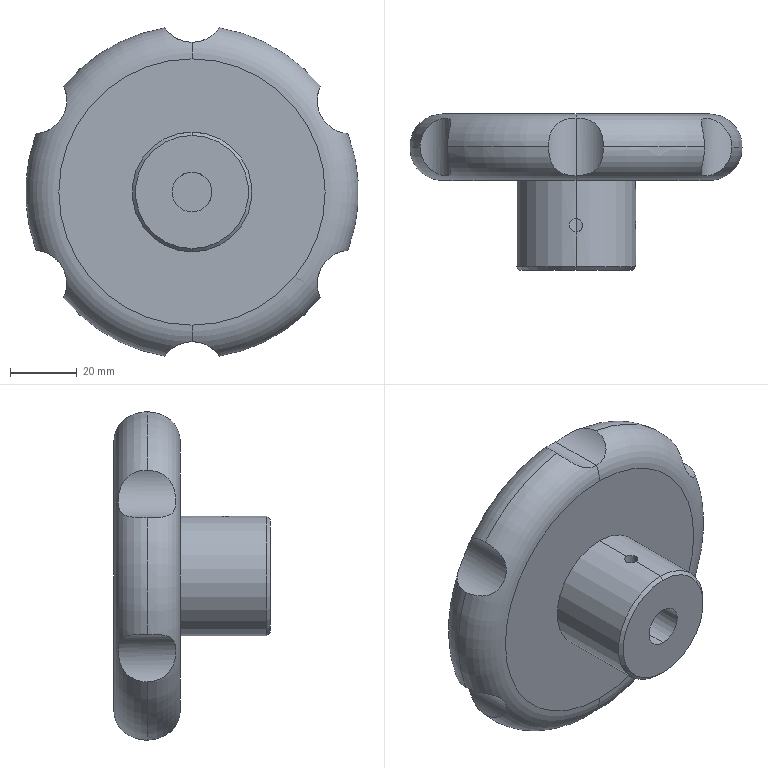Part | NX | features BREP 1 | 1 solid | 28 faces | box 100 x 47 x 98.636 mm | volume 156067 mm3 | cylinder 15 | plane 5 | cone 4 | torus 4 | commonest cylinder face diameters 20 x7 4 x4 12 x2 36 x2
STEP:
#1=CARTESIAN_POINT('',(0.,25.,6.));
#2=VERTEX_POINT('',#1);
#3=CARTESIAN_POINT('',(0.,25.,-6.));
#4=VERTEX_POINT('',#3);
#5=CARTESIAN_POINT('',(0.,25.,0.));
#6=DIRECTION('',(0.,-1.,0.));
#7=DIRECTION('',(0.,0.,1.));
#8=AXIS2_PLACEMENT_3D('',#5,#6,#7);
#9=CIRCLE('',#8,6.);
#10=EDGE_CURVE('',#2,#4,#9,.T.);
#11=ORIENTED_EDGE('',*,*,#10,.T.);
#12=CARTESIAN_POINT('',(0.,25.,0.));
#13=DIRECTION('',(0.,-1.,0.));
#14=DIRECTION('',(0.,0.,-1.));
#15=AXIS2_PLACEMENT_3D('',#12,#13,#14);
#16=CIRCLE('',#15,6.);
#17=EDGE_CURVE('',#4,#2,#16,.T.);
#18=ORIENTED_EDGE('',*,*,#17,.T.);
#19=EDGE_LOOP('',(#11,#18));
#20=FACE_BOUND('',#19,.T.);
#21=CARTESIAN_POINT('',(0.,25.,0.));
#22=DIRECTION('',(0.,1.,0.));
#23=DIRECTION('',(1.,0.,0.));
#24=AXIS2_PLACEMENT_3D('',#21,#22,#23);
#25=PLANE('',#24);
#26=ADVANCED_FACE('',(#20),#25,.F.);
#27=CARTESIAN_POINT('',(0.,0.,6.));
#28=VERTEX_POINT('',#27);
#29=CARTESIAN_POINT('',(0.,11.5,6.));
#30=VERTEX_POINT('',#29);
#31=CARTESIAN_POINT('',(0.,0.,6.));
#32=DIRECTION('',(0.,1.,0.));
#33=VECTOR('',#32,1000.);
#34=LINE('',#31,#33);
#35=EDGE_CURVE('',#28,#30,#34,.T.);
#36=ORIENTED_EDGE('',*,*,#35,.T.);
#37=CARTESIAN_POINT('',(2.,13.5,5.657));
#38=VERTEX_POINT('',#37);
#39=CARTESIAN_POINT('',(0.,11.5,6.));
#40=CARTESIAN_POINT('',(0.5281,11.5,6.));
#41=CARTESIAN_POINT('',(1.575,11.942,5.831));
#42=CARTESIAN_POINT('',(2.,12.98,5.657));
#43=CARTESIAN_POINT('',(2.,13.5,5.657));
#44=B_SPLINE_CURVE_WITH_KNOTS('',3,(#39,#40,#41,#42,#43),.UNSPECIFIED.,.F.,.F.,(4,1,4),(0.,0.5,1.),.UNSPECIFIED.);
#45=EDGE_CURVE('',#38,#30,#44,.F.);
#46=ORIENTED_EDGE('',*,*,#45,.F.);
#47=CARTESIAN_POINT('',(0.,15.5,6.));
#48=VERTEX_POINT('',#47);
#49=CARTESIAN_POINT('',(2.,13.5,5.657));
#50=CARTESIAN_POINT('',(2.,14.022,5.657));
#51=CARTESIAN_POINT('',(1.569,15.065,5.833));
#52=CARTESIAN_POINT('',(0.5245,15.5,6.));
#53=CARTESIAN_POINT('',(0.,15.5,6.));
#54=B_SPLINE_CURVE_WITH_KNOTS('',3,(#49,#50,#51,#52,#53),.UNSPECIFIED.,.F.,.F.,(4,1,4),(0.,0.5,1.),.UNSPECIFIED.);
#55=EDGE_CURVE('',#48,#38,#54,.F.);
#56=ORIENTED_EDGE('',*,*,#55,.F.);
#57=CARTESIAN_POINT('',(0.,15.5,6.));
#58=DIRECTION('',(0.,1.,0.));
#59=VECTOR('',#58,1000.);
#60=LINE('',#57,#59);
#61=EDGE_CURVE('',#2,#48,#60,.F.);
#62=ORIENTED_EDGE('',*,*,#61,.F.);
#63=ORIENTED_EDGE('',*,*,#17,.F.);
#64=CARTESIAN_POINT('',(0.,0.,-6.));
#65=VERTEX_POINT('',#64);
#66=CARTESIAN_POINT('',(0.,0.,-6.));
#67=DIRECTION('',(0.,1.,0.));
#68=VECTOR('',#67,1000.);
#69=LINE('',#66,#68);
#70=EDGE_CURVE('',#4,#65,#69,.F.);
#71=ORIENTED_EDGE('',*,*,#70,.T.);
#72=CARTESIAN_POINT('',(0.,0.,0.));
#73=DIRECTION('',(0.,1.,0.));
#74=DIRECTION('',(1.,0.,0.));
#75=AXIS2_PLACEMENT_3D('',#72,#73,#74);
#76=CIRCLE('',#75,6.);
#77=EDGE_CURVE('',#28,#65,#76,.T.);
#78=ORIENTED_EDGE('',*,*,#77,.F.);
#79=EDGE_LOOP('',(#36,#46,#56,#62,#63,#71,#78));
#80=FACE_BOUND('',#79,.T.);
#81=CARTESIAN_POINT('',(5.657,13.5,-2.));
#82=VERTEX_POINT('',#81);
#83=CARTESIAN_POINT('',(5.657,13.5,2.));
#84=VERTEX_POINT('',#83);
#85=CARTESIAN_POINT('',(5.657,13.5,2.));
#86=CARTESIAN_POINT('',(5.657,12.974,2.));
#87=CARTESIAN_POINT('',(5.836,11.924,1.555));
#88=CARTESIAN_POINT('',(6.083,11.283,0.006264));
#89=CARTESIAN_POINT('',(5.83,11.944,-1.582));
#90=CARTESIAN_POINT('',(5.657,12.981,-2.));
#91=CARTESIAN_POINT('',(5.657,13.5,-2.));
#92=B_SPLINE_CURVE_WITH_KNOTS('',3,(#85,#86,#87,#88,#89,#90,#91),.UNSPECIFIED.,.F.,.F.,(4,1,1,1,4),(0.,0.25,0.5,0.75,1.),.UNSPECIFIED.);
#93=EDGE_CURVE('',#82,#84,#92,.F.);
#94=ORIENTED_EDGE('',*,*,#93,.F.);
#95=CARTESIAN_POINT('',(5.657,13.5,-2.));
#96=CARTESIAN_POINT('',(5.657,14.,-2.));
#97=CARTESIAN_POINT('',(5.832,15.072,-1.572));
#98=CARTESIAN_POINT('',(6.083,15.714,-0.00285));
#99=CARTESIAN_POINT('',(5.834,15.071,1.564));
#100=CARTESIAN_POINT('',(5.657,14.024,2.));
#101=CARTESIAN_POINT('',(5.657,13.5,2.));
#102=B_SPLINE_CURVE_WITH_KNOTS('',3,(#95,#96,#97,#98,#99,#100,#101),.UNSPECIFIED.,.F.,.F.,(4,1,1,1,4),(0.,0.25,0.5,0.75,1.),.UNSPECIFIED.);
#103=EDGE_CURVE('',#84,#82,#102,.F.);
#104=ORIENTED_EDGE('',*,*,#103,.F.);
#105=EDGE_LOOP('',(#94,#104));
#106=FACE_BOUND('',#105,.T.);
#107=CARTESIAN_POINT('',(0.,25.,0.));
#108=DIRECTION('',(0.,1.,0.));
#109=DIRECTION('',(0.,0.,-1.));
#110=AXIS2_PLACEMENT_3D('',#107,#108,#109);
#111=CYLINDRICAL_SURFACE('',#110,6.);
#112=ADVANCED_FACE('',(#80,#106),#111,.F.);
#113=CARTESIAN_POINT('',(0.,0.,-17.));
#114=VERTEX_POINT('',#113);
#115=CARTESIAN_POINT('',(0.,0.,17.));
#116=VERTEX_POINT('',#115);
#117=CARTESIAN_POINT('',(0.,0.,0.));
#118=DIRECTION('',(0.,-1.,0.));
#119=DIRECTION('',(0.,0.,-1.));
#120=AXIS2_PLACEMENT_3D('',#117,#118,#119);
#121=CIRCLE('',#120,17.);
#122=EDGE_CURVE('',#114,#116,#121,.T.);
#123=ORIENTED_EDGE('',*,*,#122,.T.);
#124=CARTESIAN_POINT('',(0.,0.,0.));
#125=DIRECTION('',(0.,-1.,0.));
#126=DIRECTION('',(0.,0.,1.));
#127=AXIS2_PLACEMENT_3D('',#124,#125,#126);
#128=CIRCLE('',#127,17.);
#129=EDGE_CURVE('',#116,#114,#128,.T.);
#130=ORIENTED_EDGE('',*,*,#129,.T.);
#131=EDGE_LOOP('',(#123,#130));
#132=FACE_BOUND('',#131,.T.);
#133=CARTESIAN_POINT('',(0.,0.,0.));
#134=DIRECTION('',(0.,1.,0.));
#135=DIRECTION('',(0.,0.,-1.));
#136=AXIS2_PLACEMENT_3D('',#133,#134,#135);
#137=CIRCLE('',#136,6.);
#138=EDGE_CURVE('',#65,#28,#137,.T.);
#139=ORIENTED_EDGE('',*,*,#138,.T.);
#140=ORIENTED_EDGE('',*,*,#77,.T.);
#141=EDGE_LOOP('',(#139,#140));
#142=FACE_BOUND('',#141,.T.);
#143=CARTESIAN_POINT('',(0.,0.,0.));
#144=DIRECTION('',(0.,1.,0.));
#145=DIRECTION('',(1.,0.,0.));
#146=AXIS2_PLACEMENT_3D('',#143,#144,#145);
#147=PLANE('',#146);
#148=ADVANCED_FACE('',(#132,#142),#147,.F.);
#149=CARTESIAN_POINT('',(0.,1.,-18.));
#150=VERTEX_POINT('',#149);
#151=CARTESIAN_POINT('',(0.,0.,-17.));
#152=DIRECTION('',(0.,0.7071,-0.7071));
#153=VECTOR('',#152,1000.);
#154=LINE('',#151,#153);
#155=EDGE_CURVE('',#114,#150,#154,.T.);
#156=ORIENTED_EDGE('',*,*,#155,.F.);
#157=ORIENTED_EDGE('',*,*,#129,.F.);
#158=CARTESIAN_POINT('',(0.,1.,18.));
#159=VERTEX_POINT('',#158);
#160=CARTESIAN_POINT('',(0.,0.,17.));
#161=DIRECTION('',(0.,0.7071,0.7071));
#162=VECTOR('',#161,1000.);
#163=LINE('',#160,#162);
#164=EDGE_CURVE('',#116,#159,#163,.T.);
#165=ORIENTED_EDGE('',*,*,#164,.T.);
#166=CARTESIAN_POINT('',(0.,1.,0.));
#167=DIRECTION('',(0.,-1.,0.));
#168=DIRECTION('',(0.,0.,1.));
#169=AXIS2_PLACEMENT_3D('',#166,#167,#168);
#170=CIRCLE('',#169,18.);
#171=EDGE_CURVE('',#159,#150,#170,.T.);
#172=ORIENTED_EDGE('',*,*,#171,.T.);
#173=EDGE_LOOP('',(#156,#157,#165,#172));
#174=FACE_BOUND('',#173,.T.);
#175=CARTESIAN_POINT('',(0.,0.5,0.));
#176=DIRECTION('',(0.,1.,0.));
#177=DIRECTION('',(0.,0.,1.));
#178=AXIS2_PLACEMENT_3D('',#175,#176,#177);
#179=CONICAL_SURFACE('',#178,17.5,0.7854);
#180=ADVANCED_FACE('',(#174),#179,.T.);
#181=CARTESIAN_POINT('',(0.,11.5,18.));
#182=VERTEX_POINT('',#181);
#183=CARTESIAN_POINT('',(0.,11.5,18.));
#184=DIRECTION('',(0.,-1.,0.));
#185=VECTOR('',#184,1000.);
#186=LINE('',#183,#185);
#187=EDGE_CURVE('',#182,#159,#186,.T.);
#188=ORIENTED_EDGE('',*,*,#187,.F.);
#189=CARTESIAN_POINT('',(-2.,13.5,17.889));
#190=VERTEX_POINT('',#189);
#191=CARTESIAN_POINT('',(0.,11.5,18.));
#192=CARTESIAN_POINT('',(-1.065,11.5,18.));
#193=CARTESIAN_POINT('',(-1.999,12.443,17.889));
#194=CARTESIAN_POINT('',(-2.,13.5,17.889));
#195=B_SPLINE_CURVE_WITH_KNOTS('',3,(#191,#192,#193,#194),.UNSPECIFIED.,.F.,.F.,(4,4),(0.,1.),.UNSPECIFIED.);
#196=EDGE_CURVE('',#182,#190,#195,.T.);
#197=ORIENTED_EDGE('',*,*,#196,.T.);
#198=CARTESIAN_POINT('',(0.,15.5,18.));
#199=VERTEX_POINT('',#198);
#200=CARTESIAN_POINT('',(-2.,13.5,17.889));
#201=CARTESIAN_POINT('',(-1.999,14.557,17.889));
#202=CARTESIAN_POINT('',(-1.065,15.5,18.));
#203=CARTESIAN_POINT('',(0.,15.5,18.));
#204=B_SPLINE_CURVE_WITH_KNOTS('',3,(#200,#201,#202,#203),.UNSPECIFIED.,.F.,.F.,(4,4),(0.,1.),.UNSPECIFIED.);
#205=EDGE_CURVE('',#190,#199,#204,.T.);
#206=ORIENTED_EDGE('',*,*,#205,.T.);
#207=CARTESIAN_POINT('',(0.,27.,18.));
#208=VERTEX_POINT('',#207);
#209=CARTESIAN_POINT('',(0.,27.,18.));
#210=DIRECTION('',(0.,-1.,0.));
#211=VECTOR('',#210,1000.);
#212=LINE('',#209,#211);
#213=EDGE_CURVE('',#199,#208,#212,.F.);
#214=ORIENTED_EDGE('',*,*,#213,.T.);
#215=CARTESIAN_POINT('',(0.,27.,-18.));
#216=VERTEX_POINT('',#215);
#217=CARTESIAN_POINT('',(0.,27.,0.));
#218=DIRECTION('',(0.,1.,0.));
#219=DIRECTION('',(0.,0.,-1.));
#220=AXIS2_PLACEMENT_3D('',#217,#218,#219);
#221=CIRCLE('',#220,18.);
#222=EDGE_CURVE('',#216,#208,#221,.T.);
#223=ORIENTED_EDGE('',*,*,#222,.F.);
#224=CARTESIAN_POINT('',(0.,27.,-18.));
#225=DIRECTION('',(0.,-1.,0.));
#226=VECTOR('',#225,1000.);
#227=LINE('',#224,#226);
#228=EDGE_CURVE('',#150,#216,#227,.F.);
#229=ORIENTED_EDGE('',*,*,#228,.F.);
#230=ORIENTED_EDGE('',*,*,#171,.F.);
#231=EDGE_LOOP('',(#188,#197,#206,#214,#223,#229,#230));
#232=FACE_BOUND('',#231,.T.);
#233=CARTESIAN_POINT('',(0.,50.,0.));
#234=DIRECTION('',(0.,-1.,0.));
#235=DIRECTION('',(0.,0.,1.));
#236=AXIS2_PLACEMENT_3D('',#233,#234,#235);
#237=CYLINDRICAL_SURFACE('',#236,18.);
#238=ADVANCED_FACE('',(#232),#237,.T.);
#239=ORIENTED_EDGE('',*,*,#228,.T.);
#240=CARTESIAN_POINT('',(0.,27.,0.));
#241=DIRECTION('',(0.,1.,0.));
#242=DIRECTION('',(0.,0.,1.));
#243=AXIS2_PLACEMENT_3D('',#240,#241,#242);
#244=CIRCLE('',#243,18.);
#245=EDGE_CURVE('',#208,#216,#244,.T.);
#246=ORIENTED_EDGE('',*,*,#245,.F.);
#247=ORIENTED_EDGE('',*,*,#213,.F.);
#248=CARTESIAN_POINT('',(2.,13.5,17.889));
#249=VERTEX_POINT('',#248);
#250=CARTESIAN_POINT('',(0.,15.5,18.));
#251=CARTESIAN_POINT('',(1.057,15.5,18.));
#252=CARTESIAN_POINT('',(1.999,14.558,17.889));
#253=CARTESIAN_POINT('',(2.,13.5,17.889));
#254=B_SPLINE_CURVE_WITH_KNOTS('',3,(#250,#251,#252,#253),.UNSPECIFIED.,.F.,.F.,(4,4),(0.,1.),.UNSPECIFIED.);
#255=EDGE_CURVE('',#199,#249,#254,.T.);
#256=ORIENTED_EDGE('',*,*,#255,.T.);
#257=CARTESIAN_POINT('',(2.,13.5,17.889));
#258=CARTESIAN_POINT('',(1.999,12.44,17.889));
#259=CARTESIAN_POINT('',(1.061,11.5,18.));
#260=CARTESIAN_POINT('',(0.,11.5,18.));
#261=B_SPLINE_CURVE_WITH_KNOTS('',3,(#257,#258,#259,#260),.UNSPECIFIED.,.F.,.F.,(4,4),(0.,1.),.UNSPECIFIED.);
#262=EDGE_CURVE('',#249,#182,#261,.T.);
#263=ORIENTED_EDGE('',*,*,#262,.T.);
#264=ORIENTED_EDGE('',*,*,#187,.T.);
#265=CARTESIAN_POINT('',(0.,1.,0.));
#266=DIRECTION('',(0.,-1.,0.));
#267=DIRECTION('',(0.,0.,-1.));
#268=AXIS2_PLACEMENT_3D('',#265,#266,#267);
#269=CIRCLE('',#268,18.);
#270=EDGE_CURVE('',#150,#159,#269,.T.);
#271=ORIENTED_EDGE('',*,*,#270,.F.);
#272=EDGE_LOOP('',(#239,#246,#247,#256,#263,#264,#271));
#273=FACE_BOUND('',#272,.T.);
#274=CARTESIAN_POINT('',(17.889,13.5,2.));
#275=VERTEX_POINT('',#274);
#276=CARTESIAN_POINT('',(17.889,13.5,-2.));
#277=VERTEX_POINT('',#276);
#278=CARTESIAN_POINT('',(17.889,13.5,2.));
#279=CARTESIAN_POINT('',(17.889,14.03,2.));
#280=CARTESIAN_POINT('',(17.944,15.064,1.567));
#281=CARTESIAN_POINT('',(18.028,15.717,0.0006109));
#282=CARTESIAN_POINT('',(17.945,15.066,-1.564));
#283=CARTESIAN_POINT('',(17.889,14.031,-2.));
#284=CARTESIAN_POINT('',(17.889,13.5,-2.));
#285=B_SPLINE_CURVE_WITH_KNOTS('',3,(#278,#279,#280,#281,#282,#283,#284),.UNSPECIFIED.,.F.,.F.,(4,1,1,1,4),(0.,0.25,0.5,0.75,1.),.UNSPECIFIED.);
#286=EDGE_CURVE('',#275,#277,#285,.T.);
#287=ORIENTED_EDGE('',*,*,#286,.T.);
#288=CARTESIAN_POINT('',(17.889,13.5,-2.));
#289=CARTESIAN_POINT('',(17.889,12.967,-2.));
#290=CARTESIAN_POINT('',(17.945,11.93,-1.56));
#291=CARTESIAN_POINT('',(18.027,11.288,-0.005678));
#292=CARTESIAN_POINT('',(17.946,11.917,1.549));
#293=CARTESIAN_POINT('',(17.889,12.965,2.));
#294=CARTESIAN_POINT('',(17.889,13.5,2.));
#295=B_SPLINE_CURVE_WITH_KNOTS('',3,(#288,#289,#290,#291,#292,#293,#294),.UNSPECIFIED.,.F.,.F.,(4,1,1,1,4),(0.,0.25,0.5,0.75,1.),.UNSPECIFIED.);
#296=EDGE_CURVE('',#277,#275,#295,.T.);
#297=ORIENTED_EDGE('',*,*,#296,.T.);
#298=EDGE_LOOP('',(#287,#297));
#299=FACE_BOUND('',#298,.T.);
#300=CARTESIAN_POINT('',(0.,50.,0.));
#301=DIRECTION('',(0.,-1.,0.));
#302=DIRECTION('',(0.,0.,1.));
#303=AXIS2_PLACEMENT_3D('',#300,#301,#302);
#304=CYLINDRICAL_SURFACE('',#303,18.);
#305=ADVANCED_FACE('',(#273,#299),#304,.T.);
#306=ORIENTED_EDGE('',*,*,#164,.F.);
#307=ORIENTED_EDGE('',*,*,#122,.F.);
#308=ORIENTED_EDGE('',*,*,#155,.T.);
#309=ORIENTED_EDGE('',*,*,#270,.T.);
#310=EDGE_LOOP('',(#306,#307,#308,#309));
#311=FACE_BOUND('',#310,.T.);
#312=CARTESIAN_POINT('',(0.,0.5,0.));
#313=DIRECTION('',(0.,1.,0.));
#314=DIRECTION('',(0.,0.,1.));
#315=AXIS2_PLACEMENT_3D('',#312,#313,#314);
#316=CONICAL_SURFACE('',#315,17.5,0.7854);
#317=ADVANCED_FACE('',(#311),#316,.T.);
#318=CARTESIAN_POINT('',(-2.,13.5,5.657));
#319=VERTEX_POINT('',#318);
#320=CARTESIAN_POINT('',(0.,11.5,6.));
#321=CARTESIAN_POINT('',(-0.2457,11.5,6.));
#322=CARTESIAN_POINT('',(-0.6324,11.564,5.977));
#323=CARTESIAN_POINT('',(-1.071,11.805,5.905));
#324=CARTESIAN_POINT('',(-1.233,11.922,5.872));
#325=CARTESIAN_POINT('',(-1.411,12.073,5.833));
#326=CARTESIAN_POINT('',(-1.587,12.278,5.787));
#327=CARTESIAN_POINT('',(-1.68,12.408,5.76));
#328=CARTESIAN_POINT('',(-1.942,12.869,5.68));
#329=CARTESIAN_POINT('',(-2.,13.255,5.657));
#330=CARTESIAN_POINT('',(-2.,13.5,5.657));
#331=B_SPLINE_CURVE_WITH_KNOTS('',3,(#320,#321,#322,#323,#324,#325,#326,#327,#328,#329,#330),.UNSPECIFIED.,.F.,.F.,(4,1,1,1,1,1,1,1,4),(0.,0.25,0.375,0.4375,0.5,0.5625,0.625,0.75,1.),.UNSPECIFIED.);
#332=EDGE_CURVE('',#30,#319,#331,.T.);
#333=ORIENTED_EDGE('',*,*,#332,.T.);
#334=CARTESIAN_POINT('',(-2.,13.5,17.889));
#335=DIRECTION('',(0.,0.,-1.));
#336=VECTOR('',#335,1000.);
#337=LINE('',#334,#336);
#338=EDGE_CURVE('',#190,#319,#337,.T.);
#339=ORIENTED_EDGE('',*,*,#338,.F.);
#340=ORIENTED_EDGE('',*,*,#196,.F.);
#341=ORIENTED_EDGE('',*,*,#262,.F.);
#342=CARTESIAN_POINT('',(2.,13.5,17.889));
#343=DIRECTION('',(0.,0.,-1.));
#344=VECTOR('',#343,1000.);
#345=LINE('',#342,#344);
#346=EDGE_CURVE('',#249,#38,#345,.T.);
#347=ORIENTED_EDGE('',*,*,#346,.T.);
#348=ORIENTED_EDGE('',*,*,#45,.T.);
#349=EDGE_LOOP('',(#333,#339,#340,#341,#347,#348));
#350=FACE_BOUND('',#349,.T.);
#351=CARTESIAN_POINT('',(0.,13.5,18.));
#352=DIRECTION('',(0.,0.,-1.));
#353=DIRECTION('',(1.,0.,0.));
#354=AXIS2_PLACEMENT_3D('',#351,#352,#353);
#355=CYLINDRICAL_SURFACE('',#354,2.);
#356=ADVANCED_FACE('',(#350),#355,.F.);
#357=ORIENTED_EDGE('',*,*,#55,.T.);
#358=ORIENTED_EDGE('',*,*,#346,.F.);
#359=ORIENTED_EDGE('',*,*,#255,.F.);
#360=ORIENTED_EDGE('',*,*,#205,.F.);
#361=ORIENTED_EDGE('',*,*,#338,.T.);
#362=CARTESIAN_POINT('',(-2.,13.5,5.657));
#363=CARTESIAN_POINT('',(-2.,13.744,5.657));
#364=CARTESIAN_POINT('',(-1.941,14.129,5.68));
#365=CARTESIAN_POINT('',(-1.685,14.584,5.759));
#366=CARTESIAN_POINT('',(-1.589,14.719,5.786));
#367=CARTESIAN_POINT('',(-1.417,14.92,5.831));
#368=CARTESIAN_POINT('',(-1.237,15.075,5.871));
#369=CARTESIAN_POINT('',(-1.078,15.191,5.904));
#370=CARTESIAN_POINT('',(-0.637,15.435,5.977));
#371=CARTESIAN_POINT('',(-0.2473,15.5,6.));
#372=CARTESIAN_POINT('',(0.,15.5,6.));
#373=B_SPLINE_CURVE_WITH_KNOTS('',3,(#362,#363,#364,#365,#366,#367,#368,#369,#370,#371,#372),.UNSPECIFIED.,.F.,.F.,(4,1,1,1,1,1,1,1,4),(0.,0.25,0.375,0.4375,0.5,0.5625,0.625,0.75,1.),.UNSPECIFIED.);
#374=EDGE_CURVE('',#319,#48,#373,.T.);
#375=ORIENTED_EDGE('',*,*,#374,.T.);
#376=EDGE_LOOP('',(#357,#358,#359,#360,#361,#375));
#377=FACE_BOUND('',#376,.T.);
#378=CARTESIAN_POINT('',(0.,13.5,18.));
#379=DIRECTION('',(0.,0.,-1.));
#380=DIRECTION('',(1.,0.,0.));
#381=AXIS2_PLACEMENT_3D('',#378,#379,#380);
#382=CYLINDRICAL_SURFACE('',#381,2.);
#383=ADVANCED_FACE('',(#377),#382,.F.);
#384=ORIENTED_EDGE('',*,*,#138,.F.);
#385=ORIENTED_EDGE('',*,*,#70,.F.);
#386=ORIENTED_EDGE('',*,*,#10,.F.);
#387=ORIENTED_EDGE('',*,*,#61,.T.);
#388=ORIENTED_EDGE('',*,*,#374,.F.);
#389=ORIENTED_EDGE('',*,*,#332,.F.);
#390=ORIENTED_EDGE('',*,*,#35,.F.);
#391=EDGE_LOOP('',(#384,#385,#386,#387,#388,#389,#390));
#392=FACE_BOUND('',#391,.T.);
#393=CARTESIAN_POINT('',(0.,25.,0.));
#394=DIRECTION('',(0.,1.,0.));
#395=DIRECTION('',(0.,0.,-1.));
#396=AXIS2_PLACEMENT_3D('',#393,#394,#395);
#397=CYLINDRICAL_SURFACE('',#396,6.);
#398=ADVANCED_FACE('',(#392),#397,.F.);
#399=CARTESIAN_POINT('',(0.,27.,-40.));
#400=VERTEX_POINT('',#399);
#401=CARTESIAN_POINT('',(0.,27.,40.));
#402=VERTEX_POINT('',#401);
#403=CARTESIAN_POINT('',(0.,27.,0.));
#404=DIRECTION('',(0.,-1.,0.));
#405=DIRECTION('',(0.,0.,-1.));
#406=AXIS2_PLACEMENT_3D('',#403,#404,#405);
#407=CIRCLE('',#406,40.);
#408=EDGE_CURVE('',#400,#402,#407,.T.);
#409=ORIENTED_EDGE('',*,*,#408,.T.);
#410=CARTESIAN_POINT('',(0.,27.,0.));
#411=DIRECTION('',(0.,-1.,0.));
#412=DIRECTION('',(0.,0.,1.));
#413=AXIS2_PLACEMENT_3D('',#410,#411,#412);
#414=CIRCLE('',#413,40.);
#415=EDGE_CURVE('',#402,#400,#414,.T.);
#416=ORIENTED_EDGE('',*,*,#415,.T.);
#417=EDGE_LOOP('',(#409,#416));
#418=FACE_BOUND('',#417,.T.);
#419=ORIENTED_EDGE('',*,*,#222,.T.);
#420=ORIENTED_EDGE('',*,*,#245,.T.);
#421=EDGE_LOOP('',(#419,#420));
#422=FACE_BOUND('',#421,.T.);
#423=CARTESIAN_POINT('',(0.,27.,18.));
#424=DIRECTION('',(0.,1.,0.));
#425=DIRECTION('',(1.,0.,0.));
#426=AXIS2_PLACEMENT_3D('',#423,#424,#425);
#427=PLANE('',#426);
#428=ADVANCED_FACE('',(#418,#422),#427,.F.);
#429=CARTESIAN_POINT('',(0.,28.34,45.));
#430=VERTEX_POINT('',#429);
#431=CARTESIAN_POINT('',(0.,37.,40.));
#432=DIRECTION('',(-1.,0.,0.));
#433=DIRECTION('',(0.,-1.,0.));
#434=AXIS2_PLACEMENT_3D('',#431,#432,#433);
#435=CIRCLE('',#434,10.);
#436=EDGE_CURVE('',#430,#402,#435,.F.);
#437=ORIENTED_EDGE('',*,*,#436,.F.);
#438=CARTESIAN_POINT('',(-5.837,30.104,46.88));
#439=VERTEX_POINT('',#438);
#440=CARTESIAN_POINT('',(-5.837,30.104,46.88));
#441=CARTESIAN_POINT('',(-5.144,29.495,46.382));
#442=CARTESIAN_POINT('',(-3.305,28.575,45.374));
#443=CARTESIAN_POINT('',(-1.125,28.34,45.));
#444=CARTESIAN_POINT('',(0.,28.34,45.));
#445=B_SPLINE_CURVE_WITH_KNOTS('',3,(#440,#441,#442,#443,#444),.UNSPECIFIED.,.F.,.F.,(4,1,4),(0.,0.5,1.),.UNSPECIFIED.);
#446=EDGE_CURVE('',#430,#439,#445,.F.);
#447=ORIENTED_EDGE('',*,*,#446,.T.);
#448=CARTESIAN_POINT('',(-8.229,37.,49.318));
#449=VERTEX_POINT('',#448);
#450=CARTESIAN_POINT('',(-8.229,37.,49.318));
#451=CARTESIAN_POINT('',(-8.229,35.555,49.318));
#452=CARTESIAN_POINT('',(-7.84,32.733,48.706));
#453=CARTESIAN_POINT('',(-6.663,30.83,47.474));
#454=CARTESIAN_POINT('',(-5.837,30.104,46.88));
#455=B_SPLINE_CURVE_WITH_KNOTS('',3,(#450,#451,#452,#453,#454),.UNSPECIFIED.,.F.,.F.,(4,1,4),(0.,0.5,1.),.UNSPECIFIED.);
#456=EDGE_CURVE('',#449,#439,#455,.T.);
#457=ORIENTED_EDGE('',*,*,#456,.F.);
#458=CARTESIAN_POINT('',(-38.596,37.,31.786));
#459=VERTEX_POINT('',#458);
#460=CARTESIAN_POINT('',(0.,37.,0.));
#461=DIRECTION('',(0.,1.,0.));
#462=DIRECTION('',(-0.7719,0.,0.6357));
#463=AXIS2_PLACEMENT_3D('',#460,#461,#462);
#464=CIRCLE('',#463,50.);
#465=EDGE_CURVE('',#459,#449,#464,.T.);
#466=ORIENTED_EDGE('',*,*,#465,.F.);
#467=CARTESIAN_POINT('',(-43.126,29.815,18.572));
#468=VERTEX_POINT('',#467);
#469=CARTESIAN_POINT('',(-43.126,29.815,18.572));
#470=CARTESIAN_POINT('',(-42.522,29.395,18.877));
#471=CARTESIAN_POINT('',(-41.211,28.722,19.699));
#472=CARTESIAN_POINT('',(-39.414,28.292,21.596));
#473=CARTESIAN_POINT('',(-38.161,28.355,23.957));
#474=CARTESIAN_POINT('',(-37.595,28.895,26.392));
#475=CARTESIAN_POINT('',(-37.634,30.076,28.685));
#476=CARTESIAN_POINT('',(-38.009,31.785,30.348));
#477=CARTESIAN_POINT('',(-38.452,34.108,31.498));
#478=CARTESIAN_POINT('',(-38.596,36.038,31.786));
#479=CARTESIAN_POINT('',(-38.596,37.,31.786));
#480=B_SPLINE_CURVE_WITH_KNOTS('',3,(#469,#470,#471,#472,#473,#474,#475,#476,#477,#478,#479),.UNSPECIFIED.,.F.,.F.,(4,1,1,1,1,1,1,1,4),(0.,0.125,0.25,0.375,0.5,0.625,0.75,0.875,1.),.UNSPECIFIED.);
#481=EDGE_CURVE('',#468,#459,#480,.T.);
#482=ORIENTED_EDGE('',*,*,#481,.F.);
#483=CARTESIAN_POINT('',(-46.825,37.,17.533));
#484=VERTEX_POINT('',#483);
#485=CARTESIAN_POINT('',(-46.825,37.,17.533));
#486=CARTESIAN_POINT('',(-46.825,35.464,17.533));
#487=CARTESIAN_POINT('',(-46.002,32.459,17.564));
#488=CARTESIAN_POINT('',(-44.141,30.521,18.06));
#489=CARTESIAN_POINT('',(-43.126,29.815,18.572));
#490=B_SPLINE_CURVE_WITH_KNOTS('',3,(#485,#486,#487,#488,#489),.UNSPECIFIED.,.F.,.F.,(4,1,4),(0.,0.5,1.),.UNSPECIFIED.);
#491=EDGE_CURVE('',#484,#468,#490,.T.);
#492=ORIENTED_EDGE('',*,*,#491,.F.);
#493=CARTESIAN_POINT('',(-46.825,37.,-17.533));
#494=VERTEX_POINT('',#493);
#495=CARTESIAN_POINT('',(0.,37.,0.));
#496=DIRECTION('',(0.,1.,0.));
#497=DIRECTION('',(-0.9365,0.,-0.3507));
#498=AXIS2_PLACEMENT_3D('',#495,#496,#497);
#499=CIRCLE('',#498,50.);
#500=EDGE_CURVE('',#494,#484,#499,.T.);
#501=ORIENTED_EDGE('',*,*,#500,.F.);
#502=CARTESIAN_POINT('',(-37.655,29.89,-28.181));
#503=VERTEX_POINT('',#502);
#504=CARTESIAN_POINT('',(-37.655,29.89,-28.181));
#505=CARTESIAN_POINT('',(-37.61,29.464,-27.521));
#506=CARTESIAN_POINT('',(-37.635,28.956,-26.414));
#507=CARTESIAN_POINT('',(-37.974,28.541,-24.789));
#508=CARTESIAN_POINT('',(-38.603,28.303,-23.033));
#509=CARTESIAN_POINT('',(-39.491,28.327,-21.575));
#510=CARTESIAN_POINT('',(-40.693,28.613,-20.261));
#511=CARTESIAN_POINT('',(-41.903,29.052,-19.236));
#512=CARTESIAN_POINT('',(-43.614,30.037,-18.264));
#513=CARTESIAN_POINT('',(-45.258,31.745,-17.75));
#514=CARTESIAN_POINT('',(-46.497,34.078,-17.551));
#515=CARTESIAN_POINT('',(-46.825,36.028,-17.533));
#516=CARTESIAN_POINT('',(-46.825,37.,-17.533));
#517=B_SPLINE_CURVE_WITH_KNOTS('',3,(#504,#505,#506,#507,#508,#509,#510,#511,#512,#513,#514,#515,#516),.UNSPECIFIED.,.F.,.F.,(4,1,1,1,1,1,1,1,1,1,4),(0.,0.125,0.1875,0.25,0.375,0.4375,0.5,0.625,0.75,0.875,1.),.UNSPECIFIED.);
#518=EDGE_CURVE('',#503,#494,#517,.T.);
#519=ORIENTED_EDGE('',*,*,#518,.F.);
#520=CARTESIAN_POINT('',(-38.596,37.,-31.786));
#521=VERTEX_POINT('',#520);
#522=CARTESIAN_POINT('',(-38.596,37.,-31.786));
#523=CARTESIAN_POINT('',(-38.596,35.489,-31.786));
#524=CARTESIAN_POINT('',(-38.225,32.531,-31.08));
#525=CARTESIAN_POINT('',(-37.73,30.602,-29.282));
#526=CARTESIAN_POINT('',(-37.655,29.89,-28.181));
#527=B_SPLINE_CURVE_WITH_KNOTS('',3,(#522,#523,#524,#525,#526),.UNSPECIFIED.,.F.,.F.,(4,1,4),(0.,0.5,1.),.UNSPECIFIED.);
#528=EDGE_CURVE('',#521,#503,#527,.T.);
#529=ORIENTED_EDGE('',*,*,#528,.F.);
#530=CARTESIAN_POINT('',(-8.229,37.,-49.318));
#531=VERTEX_POINT('',#530);
#532=CARTESIAN_POINT('',(0.,37.,0.));
#533=DIRECTION('',(0.,1.,0.));
#534=DIRECTION('',(-0.1646,0.,-0.9864));
#535=AXIS2_PLACEMENT_3D('',#532,#533,#534);
#536=CIRCLE('',#535,50.);
#537=EDGE_CURVE('',#531,#521,#536,.T.);
#538=ORIENTED_EDGE('',*,*,#537,.F.);
#539=CARTESIAN_POINT('',(-5.837,30.104,-46.88));
#540=VERTEX_POINT('',#539);
#541=CARTESIAN_POINT('',(-5.837,30.104,-46.88));
#542=CARTESIAN_POINT('',(-6.662,30.83,-47.474));
#543=CARTESIAN_POINT('',(-7.837,32.726,-48.703));
#544=CARTESIAN_POINT('',(-8.229,35.549,-49.318));
#545=CARTESIAN_POINT('',(-8.229,37.,-49.318));
#546=B_SPLINE_CURVE_WITH_KNOTS('',3,(#541,#542,#543,#544,#545),.UNSPECIFIED.,.F.,.F.,(4,1,4),(0.,0.5,1.),.UNSPECIFIED.);
#547=EDGE_CURVE('',#540,#531,#546,.T.);
#548=ORIENTED_EDGE('',*,*,#547,.F.);
#549=CARTESIAN_POINT('',(0.,28.34,-45.));
#550=VERTEX_POINT('',#549);
#551=CARTESIAN_POINT('',(0.,28.34,-45.));
#552=CARTESIAN_POINT('',(-1.117,28.34,-45.));
#553=CARTESIAN_POINT('',(-2.721,28.509,-45.268));
#554=CARTESIAN_POINT('',(-4.718,29.268,-46.138));
#555=CARTESIAN_POINT('',(-5.489,29.799,-46.63));
#556=CARTESIAN_POINT('',(-5.837,30.104,-46.88));
#557=B_SPLINE_CURVE_WITH_KNOTS('',3,(#551,#552,#553,#554,#555,#556),.UNSPECIFIED.,.F.,.F.,(4,1,1,4),(0.,0.5,0.75,1.),.UNSPECIFIED.);
#558=EDGE_CURVE('',#540,#550,#557,.F.);
#559=ORIENTED_EDGE('',*,*,#558,.T.);
#560=CARTESIAN_POINT('',(0.,37.,-40.));
#561=DIRECTION('',(1.,0.,0.));
#562=DIRECTION('',(0.,-1.,0.));
#563=AXIS2_PLACEMENT_3D('',#560,#561,#562);
#564=CIRCLE('',#563,10.);
#565=EDGE_CURVE('',#550,#400,#564,.F.);
#566=ORIENTED_EDGE('',*,*,#565,.T.);
#567=ORIENTED_EDGE('',*,*,#415,.F.);
#568=EDGE_LOOP('',(#437,#447,#457,#466,#482,#492,#501,#519,#529,#538,#548,#559,#566,#567));
#569=FACE_BOUND('',#568,.T.);
#570=CARTESIAN_POINT('',(0.,37.,0.));
#571=DIRECTION('',(0.,1.,0.));
#572=DIRECTION('',(0.,0.,1.));
#573=AXIS2_PLACEMENT_3D('',#570,#571,#572);
#574=TOROIDAL_SURFACE('',#573,40.,10.);
#575=ADVANCED_FACE('',(#569),#574,.T.);
#576=ORIENTED_EDGE('',*,*,#565,.F.);
#577=CARTESIAN_POINT('',(8.229,37.,-49.318));
#578=VERTEX_POINT('',#577);
#579=CARTESIAN_POINT('',(8.229,37.,-49.318));
#580=CARTESIAN_POINT('',(8.229,35.65,-49.318));
#581=CARTESIAN_POINT('',(7.912,33.057,-48.809));
#582=CARTESIAN_POINT('',(6.58,30.649,-47.377));
#583=CARTESIAN_POINT('',(5.032,29.436,-46.311));
#584=CARTESIAN_POINT('',(2.977,28.547,-45.33));
#585=CARTESIAN_POINT('',(1.232,28.34,-45.));
#586=CARTESIAN_POINT('',(0.,28.34,-45.));
#587=B_SPLINE_CURVE_WITH_KNOTS('',3,(#579,#580,#581,#582,#583,#584,#585,#586),.UNSPECIFIED.,.F.,.F.,(4,1,1,1,1,4),(0.,0.25,0.5,0.625,0.75,1.),.UNSPECIFIED.);
#588=EDGE_CURVE('',#578,#550,#587,.T.);
#589=ORIENTED_EDGE('',*,*,#588,.F.);
#590=CARTESIAN_POINT('',(38.596,37.,-31.786));
#591=VERTEX_POINT('',#590);
#592=CARTESIAN_POINT('',(0.,37.,0.));
#593=DIRECTION('',(0.,1.,0.));
#594=DIRECTION('',(0.7719,0.,-0.6357));
#595=AXIS2_PLACEMENT_3D('',#592,#593,#594);
#596=CIRCLE('',#595,50.);
#597=EDGE_CURVE('',#591,#578,#596,.T.);
#598=ORIENTED_EDGE('',*,*,#597,.F.);
#599=CARTESIAN_POINT('',(37.655,29.89,-28.181));
#600=VERTEX_POINT('',#599);
#601=CARTESIAN_POINT('',(37.655,29.89,-28.181));
#602=CARTESIAN_POINT('',(37.73,30.601,-29.279));
#603=CARTESIAN_POINT('',(38.222,32.52,-31.074));
#604=CARTESIAN_POINT('',(38.596,35.484,-31.786));
#605=CARTESIAN_POINT('',(38.596,37.,-31.786));
#606=B_SPLINE_CURVE_WITH_KNOTS('',3,(#601,#602,#603,#604,#605),.UNSPECIFIED.,.F.,.F.,(4,1,4),(0.,0.5,1.),.UNSPECIFIED.);
#607=EDGE_CURVE('',#600,#591,#606,.T.);
#608=ORIENTED_EDGE('',*,*,#607,.F.);
#609=CARTESIAN_POINT('',(46.825,37.,-17.533));
#610=VERTEX_POINT('',#609);
#611=CARTESIAN_POINT('',(46.825,37.,-17.533));
#612=CARTESIAN_POINT('',(46.825,36.03,-17.533));
#613=CARTESIAN_POINT('',(46.568,34.55,-17.55));
#614=CARTESIAN_POINT('',(45.906,32.965,-17.643));
#615=CARTESIAN_POINT('',(44.99,31.463,-17.835));
#616=CARTESIAN_POINT('',(43.656,30.075,-18.249));
#617=CARTESIAN_POINT('',(41.958,29.078,-19.199));
#618=CARTESIAN_POINT('',(40.741,28.627,-20.216));
#619=CARTESIAN_POINT('',(39.528,28.331,-21.523));
#620=CARTESIAN_POINT('',(38.614,28.302,-23.014));
#621=CARTESIAN_POINT('',(37.997,28.531,-24.719));
#622=CARTESIAN_POINT('',(37.646,28.92,-26.305));
#623=CARTESIAN_POINT('',(37.608,29.452,-27.503));
#624=CARTESIAN_POINT('',(37.655,29.89,-28.181));
#625=B_SPLINE_CURVE_WITH_KNOTS('',3,(#611,#612,#613,#614,#615,#616,#617,#618,#619,#620,#621,#622,#623,#624),.UNSPECIFIED.,.F.,.F.,(4,1,1,1,1,1,1,1,1,1,1,4),(0.,0.125,0.1875,0.25,0.375,0.5,0.5625,0.625,0.75,0.8125,0.875,1.),.UNSPECIFIED.);
#626=EDGE_CURVE('',#610,#600,#625,.T.);
#627=ORIENTED_EDGE('',*,*,#626,.F.);
#628=CARTESIAN_POINT('',(46.825,37.,17.533));
#629=VERTEX_POINT('',#628);
#630=CARTESIAN_POINT('',(0.,37.,0.));
#631=DIRECTION('',(0.,1.,0.));
#632=DIRECTION('',(0.9365,0.,0.3507));
#633=AXIS2_PLACEMENT_3D('',#630,#631,#632);
#634=CIRCLE('',#633,50.);
#635=EDGE_CURVE('',#629,#610,#634,.T.);
#636=ORIENTED_EDGE('',*,*,#635,.F.);
#637=CARTESIAN_POINT('',(40.037,28.463,20.994));
#638=VERTEX_POINT('',#637);
#639=CARTESIAN_POINT('',(40.037,28.463,20.994));
#640=CARTESIAN_POINT('',(40.74,28.61,20.174));
#641=CARTESIAN_POINT('',(41.829,28.978,19.265));
#642=CARTESIAN_POINT('',(43.446,29.998,18.388));
#643=CARTESIAN_POINT('',(44.858,31.264,17.846));
#644=CARTESIAN_POINT('',(46.351,33.496,17.554));
#645=CARTESIAN_POINT('',(46.825,35.808,17.533));
#646=CARTESIAN_POINT('',(46.825,37.,17.533));
#647=B_SPLINE_CURVE_WITH_KNOTS('',3,(#639,#640,#641,#642,#643,#644,#645,#646),.UNSPECIFIED.,.F.,.F.,(4,1,1,1,1,4),(0.,0.25,0.375,0.5,0.75,1.),.UNSPECIFIED.);
#648=EDGE_CURVE('',#629,#638,#647,.F.);
#649=ORIENTED_EDGE('',*,*,#648,.T.);
#650=CARTESIAN_POINT('',(38.596,37.,31.786));
#651=VERTEX_POINT('',#650);
#652=CARTESIAN_POINT('',(38.596,37.,31.786));
#653=CARTESIAN_POINT('',(38.596,35.432,31.786));
#654=CARTESIAN_POINT('',(38.303,33.17,31.224));
#655=CARTESIAN_POINT('',(37.819,30.95,29.618));
#656=CARTESIAN_POINT('',(37.601,29.691,27.998));
#657=CARTESIAN_POINT('',(37.637,28.936,26.368));
#658=CARTESIAN_POINT('',(38.069,28.437,24.353));
#659=CARTESIAN_POINT('',(38.832,28.298,22.618));
#660=CARTESIAN_POINT('',(39.615,28.374,21.487));
#661=CARTESIAN_POINT('',(40.037,28.463,20.994));
#662=B_SPLINE_CURVE_WITH_KNOTS('',3,(#652,#653,#654,#655,#656,#657,#658,#659,#660,#661),.UNSPECIFIED.,.F.,.F.,(4,1,1,1,1,1,1,4),(0.,0.25,0.375,0.5,0.625,0.75,0.875,1.),.UNSPECIFIED.);
#663=EDGE_CURVE('',#651,#638,#662,.T.);
#664=ORIENTED_EDGE('',*,*,#663,.F.);
#665=CARTESIAN_POINT('',(8.229,37.,49.318));
#666=VERTEX_POINT('',#665);
#667=CARTESIAN_POINT('',(0.,37.,0.));
#668=DIRECTION('',(0.,1.,0.));
#669=DIRECTION('',(0.1646,0.,0.9864));
#670=AXIS2_PLACEMENT_3D('',#667,#668,#669);
#671=CIRCLE('',#670,50.);
#672=EDGE_CURVE('',#666,#651,#671,.T.);
#673=ORIENTED_EDGE('',*,*,#672,.F.);
#674=CARTESIAN_POINT('',(0.,28.34,45.));
#675=CARTESIAN_POINT('',(1.267,28.34,45.));
#676=CARTESIAN_POINT('',(2.968,28.546,45.329));
#677=CARTESIAN_POINT('',(5.038,29.438,46.314));
#678=CARTESIAN_POINT('',(6.186,30.339,47.106));
#679=CARTESIAN_POINT('',(7.15,31.648,47.978));
#680=CARTESIAN_POINT('',(7.759,33.156,48.676));
#681=CARTESIAN_POINT('',(8.156,35.045,49.208));
#682=CARTESIAN_POINT('',(8.229,36.331,49.318));
#683=CARTESIAN_POINT('',(8.229,37.,49.318));
#684=B_SPLINE_CURVE_WITH_KNOTS('',3,(#674,#675,#676,#677,#678,#679,#680,#681,#682,#683),.UNSPECIFIED.,.F.,.F.,(4,1,1,1,1,1,1,4),(0.,0.25,0.375,0.5,0.625,0.75,0.875,1.),.UNSPECIFIED.);
#685=EDGE_CURVE('',#430,#666,#684,.T.);
#686=ORIENTED_EDGE('',*,*,#685,.F.);
#687=ORIENTED_EDGE('',*,*,#436,.T.);
#688=ORIENTED_EDGE('',*,*,#408,.F.);
#689=EDGE_LOOP('',(#576,#589,#598,#608,#627,#636,#649,#664,#673,#686,#687,#688));
#690=FACE_BOUND('',#689,.T.);
#691=CARTESIAN_POINT('',(0.,37.,0.));
#692=DIRECTION('',(0.,1.,0.));
#693=DIRECTION('',(0.,0.,1.));
#694=AXIS2_PLACEMENT_3D('',#691,#692,#693);
#695=TOROIDAL_SURFACE('',#694,40.,10.);
#696=ADVANCED_FACE('',(#690),#695,.T.);
#697=CARTESIAN_POINT('',(0.,45.66,45.));
#698=VERTEX_POINT('',#697);
#699=CARTESIAN_POINT('',(0.,47.,45.));
#700=DIRECTION('',(0.,1.,0.));
#701=VECTOR('',#700,1000.);
#702=LINE('',#699,#701);
#703=EDGE_CURVE('',#430,#698,#702,.T.);
#704=ORIENTED_EDGE('',*,*,#703,.F.);
#705=ORIENTED_EDGE('',*,*,#685,.T.);
#706=CARTESIAN_POINT('',(8.229,37.,49.318));
#707=CARTESIAN_POINT('',(8.229,38.361,49.318));
#708=CARTESIAN_POINT('',(7.903,40.999,48.793));
#709=CARTESIAN_POINT('',(6.546,43.388,47.348));
#710=CARTESIAN_POINT('',(5.002,44.581,46.294));
#711=CARTESIAN_POINT('',(2.95,45.458,45.323));
#712=CARTESIAN_POINT('',(1.22,45.66,45.));
#713=CARTESIAN_POINT('',(0.,45.66,45.));
#714=B_SPLINE_CURVE_WITH_KNOTS('',3,(#706,#707,#708,#709,#710,#711,#712,#713),.UNSPECIFIED.,.F.,.F.,(4,1,1,1,1,4),(0.,0.25,0.5,0.625,0.75,1.),.UNSPECIFIED.);
#715=EDGE_CURVE('',#666,#698,#714,.T.);
#716=ORIENTED_EDGE('',*,*,#715,.T.);
#717=EDGE_LOOP('',(#704,#705,#716));
#718=FACE_BOUND('',#717,.T.);
#719=CARTESIAN_POINT('',(0.,47.,55.));
#720=DIRECTION('',(0.,1.,0.));
#721=DIRECTION('',(0.,0.,-1.));
#722=AXIS2_PLACEMENT_3D('',#719,#720,#721);
#723=CYLINDRICAL_SURFACE('',#722,10.);
#724=ADVANCED_FACE('',(#718),#723,.F.);
#725=CARTESIAN_POINT('',(0.,45.66,-45.));
#726=VERTEX_POINT('',#725);
#727=CARTESIAN_POINT('',(0.,47.,-40.));
#728=VERTEX_POINT('',#727);
#729=CARTESIAN_POINT('',(0.,37.,-40.));
#730=DIRECTION('',(1.,0.,0.));
#731=DIRECTION('',(0.,0.866,-0.5));
#732=AXIS2_PLACEMENT_3D('',#729,#730,#731);
#733=CIRCLE('',#732,10.);
#734=EDGE_CURVE('',#726,#728,#733,.T.);
#735=ORIENTED_EDGE('',*,*,#734,.F.);
#736=CARTESIAN_POINT('',(-8.229,37.,-49.318));
#737=CARTESIAN_POINT('',(-8.229,38.344,-49.318));
#738=CARTESIAN_POINT('',(-7.915,40.938,-48.813));
#739=CARTESIAN_POINT('',(-6.58,43.351,-47.377));
#740=CARTESIAN_POINT('',(-5.03,44.566,-46.309));
#741=CARTESIAN_POINT('',(-2.966,45.456,-45.327));
#742=CARTESIAN_POINT('',(-1.227,45.66,-45.));
#743=CARTESIAN_POINT('',(0.,45.66,-45.));
#744=B_SPLINE_CURVE_WITH_KNOTS('',3,(#736,#737,#738,#739,#740,#741,#742,#743),.UNSPECIFIED.,.F.,.F.,(4,1,1,1,1,4),(0.,0.25,0.5,0.625,0.75,1.),.UNSPECIFIED.);
#745=EDGE_CURVE('',#531,#726,#744,.T.);
#746=ORIENTED_EDGE('',*,*,#745,.F.);
#747=ORIENTED_EDGE('',*,*,#537,.T.);
#748=CARTESIAN_POINT('',(-46.825,37.,-17.533));
#749=CARTESIAN_POINT('',(-46.825,38.364,-17.533));
#750=CARTESIAN_POINT('',(-46.333,40.36,-17.56));
#751=CARTESIAN_POINT('',(-45.112,42.364,-17.801));
#752=CARTESIAN_POINT('',(-43.899,43.65,-18.191));
#753=CARTESIAN_POINT('',(-42.621,44.566,-18.797));
#754=CARTESIAN_POINT('',(-41.196,45.241,-19.779));
#755=CARTESIAN_POINT('',(-39.957,45.586,-21.006));
#756=CARTESIAN_POINT('',(-38.547,45.734,-23.014));
#757=CARTESIAN_POINT('',(-37.758,45.441,-25.291));
#758=CARTESIAN_POINT('',(-37.591,44.55,-27.543));
#759=CARTESIAN_POINT('',(-37.746,43.318,-29.418));
#760=CARTESIAN_POINT('',(-38.305,40.989,-31.228));
#761=CARTESIAN_POINT('',(-38.596,38.361,-31.786));
#762=CARTESIAN_POINT('',(-38.596,37.,-31.786));
#763=B_SPLINE_CURVE_WITH_KNOTS('',3,(#748,#749,#750,#751,#752,#753,#754,#755,#756,#757,#758,#759,#760,#761,#762),.UNSPECIFIED.,.F.,.F.,(4,1,1,1,1,1,1,1,1,1,1,1,4),(0.,0.125,0.1875,0.25,0.3125,0.375,0.4375,0.5,0.625,0.6875,0.75,0.875,1.),.UNSPECIFIED.);
#764=EDGE_CURVE('',#494,#521,#763,.T.);
#765=ORIENTED_EDGE('',*,*,#764,.F.);
#766=ORIENTED_EDGE('',*,*,#500,.T.);
#767=CARTESIAN_POINT('',(-38.596,37.,31.786));
#768=CARTESIAN_POINT('',(-38.596,38.365,31.785));
#769=CARTESIAN_POINT('',(-38.304,40.996,31.226));
#770=CARTESIAN_POINT('',(-37.743,43.33,29.407));
#771=CARTESIAN_POINT('',(-37.589,44.567,27.513));
#772=CARTESIAN_POINT('',(-37.727,45.239,25.792));
#773=CARTESIAN_POINT('',(-38.168,45.586,24.109));
#774=CARTESIAN_POINT('',(-39.201,45.735,21.881));
#775=CARTESIAN_POINT('',(-40.774,45.444,20.061));
#776=CARTESIAN_POINT('',(-42.641,44.554,18.788));
#777=CARTESIAN_POINT('',(-44.343,43.325,17.982));
#778=CARTESIAN_POINT('',(-46.199,40.989,17.558));
#779=CARTESIAN_POINT('',(-46.825,38.36,17.533));
#780=CARTESIAN_POINT('',(-46.825,37.,17.533));
#781=B_SPLINE_CURVE_WITH_KNOTS('',3,(#767,#768,#769,#770,#771,#772,#773,#774,#775,#776,#777,#778,#779,#780),.UNSPECIFIED.,.F.,.F.,(4,1,1,1,1,1,1,1,1,1,1,4),(0.,0.125,0.25,0.3125,0.375,0.4375,0.5,0.625,0.6875,0.75,0.875,1.),.UNSPECIFIED.);
#782=EDGE_CURVE('',#459,#484,#781,.T.);
#783=ORIENTED_EDGE('',*,*,#782,.F.);
#784=ORIENTED_EDGE('',*,*,#465,.T.);
#785=CARTESIAN_POINT('',(0.,45.66,45.));
#786=CARTESIAN_POINT('',(-1.238,45.661,45.));
#787=CARTESIAN_POINT('',(-3.607,45.366,45.461));
#788=CARTESIAN_POINT('',(-6.385,43.79,47.133));
#789=CARTESIAN_POINT('',(-7.909,40.907,48.817));
#790=CARTESIAN_POINT('',(-8.229,38.335,49.318));
#791=CARTESIAN_POINT('',(-8.229,37.,49.318));
#792=B_SPLINE_CURVE_WITH_KNOTS('',3,(#785,#786,#787,#788,#789,#790,#791),.UNSPECIFIED.,.F.,.F.,(4,1,1,1,4),(0.,0.25,0.5,0.75,1.),.UNSPECIFIED.);
#793=EDGE_CURVE('',#698,#449,#792,.T.);
#794=ORIENTED_EDGE('',*,*,#793,.F.);
#795=CARTESIAN_POINT('',(0.,47.,40.));
#796=VERTEX_POINT('',#795);
#797=CARTESIAN_POINT('',(0.,37.,40.));
#798=DIRECTION('',(-1.,0.,0.));
#799=DIRECTION('',(0.,0.866,0.5));
#800=AXIS2_PLACEMENT_3D('',#797,#798,#799);
#801=CIRCLE('',#800,10.);
#802=EDGE_CURVE('',#698,#796,#801,.T.);
#803=ORIENTED_EDGE('',*,*,#802,.T.);
#804=CARTESIAN_POINT('',(0.,47.,0.));
#805=DIRECTION('',(0.,1.,0.));
#806=DIRECTION('',(0.,0.,-1.));
#807=AXIS2_PLACEMENT_3D('',#804,#805,#806);
#808=CIRCLE('',#807,40.);
#809=EDGE_CURVE('',#728,#796,#808,.T.);
#810=ORIENTED_EDGE('',*,*,#809,.F.);
#811=EDGE_LOOP('',(#735,#746,#747,#765,#766,#783,#784,#794,#803,#810));
#812=FACE_BOUND('',#811,.T.);
#813=CARTESIAN_POINT('',(0.,37.,0.));
#814=DIRECTION('',(0.,1.,0.));
#815=DIRECTION('',(0.,0.,1.));
#816=AXIS2_PLACEMENT_3D('',#813,#814,#815);
#817=TOROIDAL_SURFACE('',#816,40.,10.);
#818=ADVANCED_FACE('',(#812),#817,.T.);
#819=ORIENTED_EDGE('',*,*,#809,.T.);
#820=CARTESIAN_POINT('',(0.,47.,0.));
#821=DIRECTION('',(0.,1.,0.));
#822=DIRECTION('',(0.,0.,1.));
#823=AXIS2_PLACEMENT_3D('',#820,#821,#822);
#824=CIRCLE('',#823,40.);
#825=EDGE_CURVE('',#796,#728,#824,.T.);
#826=ORIENTED_EDGE('',*,*,#825,.T.);
#827=EDGE_LOOP('',(#819,#826));
#828=FACE_BOUND('',#827,.T.);
#829=CARTESIAN_POINT('',(0.,47.,-38.));
#830=VERTEX_POINT('',#829);
#831=CARTESIAN_POINT('',(0.,47.,38.));
#832=VERTEX_POINT('',#831);
#833=CARTESIAN_POINT('',(0.,47.,0.));
#834=DIRECTION('',(0.,-1.,0.));
#835=DIRECTION('',(0.,0.,-1.));
#836=AXIS2_PLACEMENT_3D('',#833,#834,#835);
#837=CIRCLE('',#836,38.);
#838=EDGE_CURVE('',#830,#832,#837,.T.);
#839=ORIENTED_EDGE('',*,*,#838,.T.);
#840=CARTESIAN_POINT('',(0.,47.,0.));
#841=DIRECTION('',(0.,-1.,0.));
#842=DIRECTION('',(0.,0.,1.));
#843=AXIS2_PLACEMENT_3D('',#840,#841,#842);
#844=CIRCLE('',#843,38.);
#845=EDGE_CURVE('',#832,#830,#844,.T.);
#846=ORIENTED_EDGE('',*,*,#845,.T.);
#847=EDGE_LOOP('',(#839,#846));
#848=FACE_BOUND('',#847,.T.);
#849=CARTESIAN_POINT('',(0.,47.,40.));
#850=DIRECTION('',(0.,-1.,0.));
#851=DIRECTION('',(0.,0.,-1.));
#852=AXIS2_PLACEMENT_3D('',#849,#850,#851);
#853=PLANE('',#852);
#854=ADVANCED_FACE('',(#828,#848),#853,.F.);
#855=ORIENTED_EDGE('',*,*,#802,.F.);
#856=ORIENTED_EDGE('',*,*,#715,.F.);
#857=ORIENTED_EDGE('',*,*,#672,.T.);
#858=CARTESIAN_POINT('',(46.825,37.,17.533));
#859=CARTESIAN_POINT('',(46.825,38.402,17.533));
#860=CARTESIAN_POINT('',(46.295,40.464,17.564));
#861=CARTESIAN_POINT('',(45.038,42.465,17.817));
#862=CARTESIAN_POINT('',(43.769,43.76,18.244));
#863=CARTESIAN_POINT('',(42.524,44.621,18.853));
#864=CARTESIAN_POINT('',(41.09,45.276,19.873));
#865=CARTESIAN_POINT('',(39.97,45.581,21.003));
#866=CARTESIAN_POINT('',(38.913,45.7,22.483));
#867=CARTESIAN_POINT('',(38.166,45.578,24.136));
#868=CARTESIAN_POINT('',(37.751,45.268,25.674));
#869=CARTESIAN_POINT('',(37.589,44.611,27.42));
#870=CARTESIAN_POINT('',(37.687,43.747,28.8));
#871=CARTESIAN_POINT('',(37.952,42.452,30.105));
#872=CARTESIAN_POINT('',(38.36,40.452,31.315));
#873=CARTESIAN_POINT('',(38.596,38.394,31.786));
#874=CARTESIAN_POINT('',(38.596,37.,31.786));
#875=B_SPLINE_CURVE_WITH_KNOTS('',3,(#858,#859,#860,#861,#862,#863,#864,#865,#866,#867,#868,#869,#870,#871,#872,#873,#874),.UNSPECIFIED.,.F.,.F.,(4,1,1,1,1,1,1,1,1,1,1,1,1,1,4),(0.,0.125,0.1875,0.25,0.3125,0.375,0.4375,0.5,0.5625,0.625,0.6875,0.75,0.8125,0.875,1.),.UNSPECIFIED.);
#876=EDGE_CURVE('',#651,#629,#875,.F.);
#877=ORIENTED_EDGE('',*,*,#876,.T.);
#878=ORIENTED_EDGE('',*,*,#635,.T.);
#879=CARTESIAN_POINT('',(38.596,37.,-31.786));
#880=CARTESIAN_POINT('',(38.596,38.348,-31.786));
#881=CARTESIAN_POINT('',(38.378,40.335,-31.355));
#882=CARTESIAN_POINT('',(37.975,42.347,-30.18));
#883=CARTESIAN_POINT('',(37.706,43.637,-28.937));
#884=CARTESIAN_POINT('',(37.59,44.555,-27.533));
#885=CARTESIAN_POINT('',(37.768,45.454,-25.243));
#886=CARTESIAN_POINT('',(38.547,45.738,-22.998));
#887=CARTESIAN_POINT('',(40.018,45.577,-20.935));
#888=CARTESIAN_POINT('',(41.211,45.232,-19.771));
#889=CARTESIAN_POINT('',(42.632,44.562,-18.79));
#890=CARTESIAN_POINT('',(44.333,43.333,-17.987));
#891=CARTESIAN_POINT('',(46.186,41.013,-17.559));
#892=CARTESIAN_POINT('',(46.825,38.375,-17.533));
#893=CARTESIAN_POINT('',(46.825,37.,-17.533));
#894=B_SPLINE_CURVE_WITH_KNOTS('',3,(#879,#880,#881,#882,#883,#884,#885,#886,#887,#888,#889,#890,#891,#892,#893),.UNSPECIFIED.,.F.,.F.,(4,1,1,1,1,1,1,1,1,1,1,1,4),(0.,0.125,0.1875,0.25,0.3125,0.375,0.5,0.5625,0.625,0.6875,0.75,0.875,1.),.UNSPECIFIED.);
#895=EDGE_CURVE('',#591,#610,#894,.T.);
#896=ORIENTED_EDGE('',*,*,#895,.F.);
#897=ORIENTED_EDGE('',*,*,#597,.T.);
#898=CARTESIAN_POINT('',(0.,45.66,-45.));
#899=CARTESIAN_POINT('',(1.256,45.66,-45.));
#900=CARTESIAN_POINT('',(3.034,45.443,-45.346));
#901=CARTESIAN_POINT('',(5.095,44.53,-46.347));
#902=CARTESIAN_POINT('',(6.649,43.272,-47.437));
#903=CARTESIAN_POINT('',(7.929,40.848,-48.839));
#904=CARTESIAN_POINT('',(8.229,38.311,-49.318));
#905=CARTESIAN_POINT('',(8.229,37.,-49.318));
#906=B_SPLINE_CURVE_WITH_KNOTS('',3,(#898,#899,#900,#901,#902,#903,#904,#905),.UNSPECIFIED.,.F.,.F.,(4,1,1,1,1,4),(0.,0.25,0.375,0.5,0.75,1.),.UNSPECIFIED.);
#907=EDGE_CURVE('',#726,#578,#906,.T.);
#908=ORIENTED_EDGE('',*,*,#907,.F.);
#909=ORIENTED_EDGE('',*,*,#734,.T.);
#910=ORIENTED_EDGE('',*,*,#825,.F.);
#911=EDGE_LOOP('',(#855,#856,#857,#877,#878,#896,#897,#908,#909,#910));
#912=FACE_BOUND('',#911,.T.);
#913=CARTESIAN_POINT('',(0.,37.,0.));
#914=DIRECTION('',(0.,1.,0.));
#915=DIRECTION('',(0.,0.,1.));
#916=AXIS2_PLACEMENT_3D('',#913,#914,#915);
#917=TOROIDAL_SURFACE('',#916,40.,10.);
#918=ADVANCED_FACE('',(#912),#917,.T.);
#919=ORIENTED_EDGE('',*,*,#745,.T.);
#920=ORIENTED_EDGE('',*,*,#907,.T.);
#921=ORIENTED_EDGE('',*,*,#588,.T.);
#922=ORIENTED_EDGE('',*,*,#558,.F.);
#923=ORIENTED_EDGE('',*,*,#547,.T.);
#924=EDGE_LOOP('',(#919,#920,#921,#922,#923));
#925=FACE_BOUND('',#924,.T.);
#926=CARTESIAN_POINT('',(0.,47.,-55.));
#927=DIRECTION('',(0.,1.,0.));
#928=DIRECTION('',(0.,0.,-1.));
#929=AXIS2_PLACEMENT_3D('',#926,#927,#928);
#930=CYLINDRICAL_SURFACE('',#929,10.);
#931=ADVANCED_FACE('',(#925),#930,.F.);
#932=ORIENTED_EDGE('',*,*,#895,.T.);
#933=ORIENTED_EDGE('',*,*,#626,.T.);
#934=ORIENTED_EDGE('',*,*,#607,.T.);
#935=EDGE_LOOP('',(#932,#933,#934));
#936=FACE_BOUND('',#935,.T.);
#937=CARTESIAN_POINT('',(47.631,47.,-27.5));
#938=DIRECTION('',(0.,1.,0.));
#939=DIRECTION('',(0.,0.,-1.));
#940=AXIS2_PLACEMENT_3D('',#937,#938,#939);
#941=CYLINDRICAL_SURFACE('',#940,10.);
#942=ADVANCED_FACE('',(#936),#941,.F.);
#943=ORIENTED_EDGE('',*,*,#876,.F.);
#944=ORIENTED_EDGE('',*,*,#663,.T.);
#945=ORIENTED_EDGE('',*,*,#648,.F.);
#946=EDGE_LOOP('',(#943,#944,#945));
#947=FACE_BOUND('',#946,.T.);
#948=CARTESIAN_POINT('',(47.631,47.,27.5));
#949=DIRECTION('',(0.,1.,0.));
#950=DIRECTION('',(0.,0.,-1.));
#951=AXIS2_PLACEMENT_3D('',#948,#949,#950);
#952=CYLINDRICAL_SURFACE('',#951,10.);
#953=ADVANCED_FACE('',(#947),#952,.F.);
#954=CARTESIAN_POINT('',(0.,45.,36.));
#955=VERTEX_POINT('',#954);
#956=CARTESIAN_POINT('',(0.,45.,36.));
#957=DIRECTION('',(0.,0.7071,0.7071));
#958=VECTOR('',#957,1000.);
#959=LINE('',#956,#958);
#960=EDGE_CURVE('',#832,#955,#959,.F.);
#961=ORIENTED_EDGE('',*,*,#960,.T.);
#962=CARTESIAN_POINT('',(0.,45.,-36.));
#963=VERTEX_POINT('',#962);
#964=CARTESIAN_POINT('',(0.,45.,0.));
#965=DIRECTION('',(0.,1.,0.));
#966=DIRECTION('',(0.,0.,-1.));
#967=AXIS2_PLACEMENT_3D('',#964,#965,#966);
#968=CIRCLE('',#967,36.);
#969=EDGE_CURVE('',#963,#955,#968,.T.);
#970=ORIENTED_EDGE('',*,*,#969,.F.);
#971=CARTESIAN_POINT('',(0.,45.,-36.));
#972=DIRECTION('',(0.,0.7071,-0.7071));
#973=VECTOR('',#972,1000.);
#974=LINE('',#971,#973);
#975=EDGE_CURVE('',#830,#963,#974,.F.);
#976=ORIENTED_EDGE('',*,*,#975,.F.);
#977=ORIENTED_EDGE('',*,*,#845,.F.);
#978=EDGE_LOOP('',(#961,#970,#976,#977));
#979=FACE_BOUND('',#978,.T.);
#980=CARTESIAN_POINT('',(0.,46.,0.));
#981=DIRECTION('',(0.,1.,0.));
#982=DIRECTION('',(0.,0.,1.));
#983=AXIS2_PLACEMENT_3D('',#980,#981,#982);
#984=CONICAL_SURFACE('',#983,37.,0.7854);
#985=ADVANCED_FACE('',(#979),#984,.F.);
#986=ORIENTED_EDGE('',*,*,#975,.T.);
#987=CARTESIAN_POINT('',(0.,45.,0.));
#988=DIRECTION('',(0.,1.,0.));
#989=DIRECTION('',(0.,0.,1.));
#990=AXIS2_PLACEMENT_3D('',#987,#988,#989);
#991=CIRCLE('',#990,36.);
#992=EDGE_CURVE('',#955,#963,#991,.T.);
#993=ORIENTED_EDGE('',*,*,#992,.F.);
#994=ORIENTED_EDGE('',*,*,#960,.F.);
#995=ORIENTED_EDGE('',*,*,#838,.F.);
#996=EDGE_LOOP('',(#986,#993,#994,#995));
#997=FACE_BOUND('',#996,.T.);
#998=CARTESIAN_POINT('',(0.,46.,0.));
#999=DIRECTION('',(0.,1.,0.));
#1000=DIRECTION('',(0.,0.,1.));
#1001=AXIS2_PLACEMENT_3D('',#998,#999,#1000);
#1002=CONICAL_SURFACE('',#1001,37.,0.7854);
#1003=ADVANCED_FACE('',(#997),#1002,.F.);
#1004=ORIENTED_EDGE('',*,*,#969,.T.);
#1005=ORIENTED_EDGE('',*,*,#992,.T.);
#1006=EDGE_LOOP('',(#1004,#1005));
#1007=FACE_BOUND('',#1006,.T.);
#1008=CARTESIAN_POINT('',(0.,45.,36.));
#1009=DIRECTION('',(0.,-1.,0.));
#1010=DIRECTION('',(0.,0.,-1.));
#1011=AXIS2_PLACEMENT_3D('',#1008,#1009,#1010);
#1012=PLANE('',#1011);
#1013=ADVANCED_FACE('',(#1007),#1012,.F.);
#1014=ORIENTED_EDGE('',*,*,#782,.T.);
#1015=ORIENTED_EDGE('',*,*,#491,.T.);
#1016=ORIENTED_EDGE('',*,*,#481,.T.);
#1017=EDGE_LOOP('',(#1014,#1015,#1016));
#1018=FACE_BOUND('',#1017,.T.);
#1019=CARTESIAN_POINT('',(-47.631,47.,27.5));
#1020=DIRECTION('',(0.,1.,0.));
#1021=DIRECTION('',(0.,0.,-1.));
#1022=AXIS2_PLACEMENT_3D('',#1019,#1020,#1021);
#1023=CYLINDRICAL_SURFACE('',#1022,10.);
#1024=ADVANCED_FACE('',(#1018),#1023,.F.);
#1025=ORIENTED_EDGE('',*,*,#764,.T.);
#1026=ORIENTED_EDGE('',*,*,#528,.T.);
#1027=ORIENTED_EDGE('',*,*,#518,.T.);
#1028=EDGE_LOOP('',(#1025,#1026,#1027));
#1029=FACE_BOUND('',#1028,.T.);
#1030=CARTESIAN_POINT('',(-47.631,47.,-27.5));
#1031=DIRECTION('',(0.,1.,0.));
#1032=DIRECTION('',(0.,0.,-1.));
#1033=AXIS2_PLACEMENT_3D('',#1030,#1031,#1032);
#1034=CYLINDRICAL_SURFACE('',#1033,10.);
#1035=ADVANCED_FACE('',(#1029),#1034,.F.);
#1036=CARTESIAN_POINT('',(17.889,13.5,2.));
#1037=CARTESIAN_POINT('',(13.811,13.5,2.));
#1038=CARTESIAN_POINT('',(9.734,13.5,2.));
#1039=CARTESIAN_POINT('',(5.657,13.5,2.));
#1040=B_SPLINE_CURVE_WITH_KNOTS('',3,(#1036,#1037,#1038,#1039),.UNSPECIFIED.,.F.,.F.,(4,4),(0.,1.),.UNSPECIFIED.);
#1041=EDGE_CURVE('',#275,#84,#1040,.T.);
#1042=ORIENTED_EDGE('',*,*,#1041,.F.);
#1043=ORIENTED_EDGE('',*,*,#296,.F.);
#1044=CARTESIAN_POINT('',(17.889,13.5,-2.));
#1045=DIRECTION('',(-1.,0.,0.));
#1046=VECTOR('',#1045,1000.);
#1047=LINE('',#1044,#1046);
#1048=EDGE_CURVE('',#277,#82,#1047,.T.);
#1049=ORIENTED_EDGE('',*,*,#1048,.T.);
#1050=ORIENTED_EDGE('',*,*,#93,.T.);
#1051=EDGE_LOOP('',(#1042,#1043,#1049,#1050));
#1052=FACE_BOUND('',#1051,.T.);
#1053=CARTESIAN_POINT('',(18.,13.5,0.));
#1054=DIRECTION('',(-1.,0.,0.));
#1055=DIRECTION('',(0.,0.,-1.));
#1056=AXIS2_PLACEMENT_3D('',#1053,#1054,#1055);
#1057=CYLINDRICAL_SURFACE('',#1056,2.);
#1058=ADVANCED_FACE('',(#1052),#1057,.F.);
#1059=ORIENTED_EDGE('',*,*,#1048,.F.);
#1060=ORIENTED_EDGE('',*,*,#286,.F.);
#1061=ORIENTED_EDGE('',*,*,#1041,.T.);
#1062=ORIENTED_EDGE('',*,*,#103,.T.);
#1063=EDGE_LOOP('',(#1059,#1060,#1061,#1062));
#1064=FACE_BOUND('',#1063,.T.);
#1065=CARTESIAN_POINT('',(18.,13.5,0.));
#1066=DIRECTION('',(-1.,0.,0.));
#1067=DIRECTION('',(0.,0.,-1.));
#1068=AXIS2_PLACEMENT_3D('',#1065,#1066,#1067);
#1069=CYLINDRICAL_SURFACE('',#1068,2.);
#1070=ADVANCED_FACE('',(#1064),#1069,.F.);
#1071=ORIENTED_EDGE('',*,*,#446,.F.);
#1072=ORIENTED_EDGE('',*,*,#703,.T.);
#1073=ORIENTED_EDGE('',*,*,#793,.T.);
#1074=ORIENTED_EDGE('',*,*,#456,.T.);
#1075=EDGE_LOOP('',(#1071,#1072,#1073,#1074));
#1076=FACE_BOUND('',#1075,.T.);
#1077=CARTESIAN_POINT('',(0.,47.,55.));
#1078=DIRECTION('',(0.,1.,0.));
#1079=DIRECTION('',(0.,0.,-1.));
#1080=AXIS2_PLACEMENT_3D('',#1077,#1078,#1079);
#1081=CYLINDRICAL_SURFACE('',#1080,10.);
#1082=ADVANCED_FACE('',(#1076),#1081,.F.);
#1083=CLOSED_SHELL('',(#26,#112,#148,#180,#238,#305,#317,#356,#383,#398,#428,#575,#696,#724,#818,#854,#918,#931,#942,#953,#985,#1003,#1013,#1024,#1035,#1058,#1070,#1082));
#1084=MANIFOLD_SOLID_BREP('',#1083);
#1085=(LENGTH_UNIT()NAMED_UNIT(*)SI_UNIT(.MILLI.,.METRE.));
#1086=UNCERTAINTY_MEASURE_WITH_UNIT(LENGTH_MEASURE(0.0508),#1085,'','');
#1087=(NAMED_UNIT(*)PLANE_ANGLE_UNIT()SI_UNIT($,.RADIAN.));
#1088=(NAMED_UNIT(*)SI_UNIT($,.STERADIAN.)SOLID_ANGLE_UNIT());
#1089=(GEOMETRIC_REPRESENTATION_CONTEXT(3)GLOBAL_UNCERTAINTY_ASSIGNED_CONTEXT((#1086))GLOBAL_UNIT_ASSIGNED_CONTEXT((#1085,#1087,#1088))REPRESENTATION_CONTEXT('',''));
#1090=ADVANCED_BREP_SHAPE_REPRESENTATION('',(#1084),#1089);